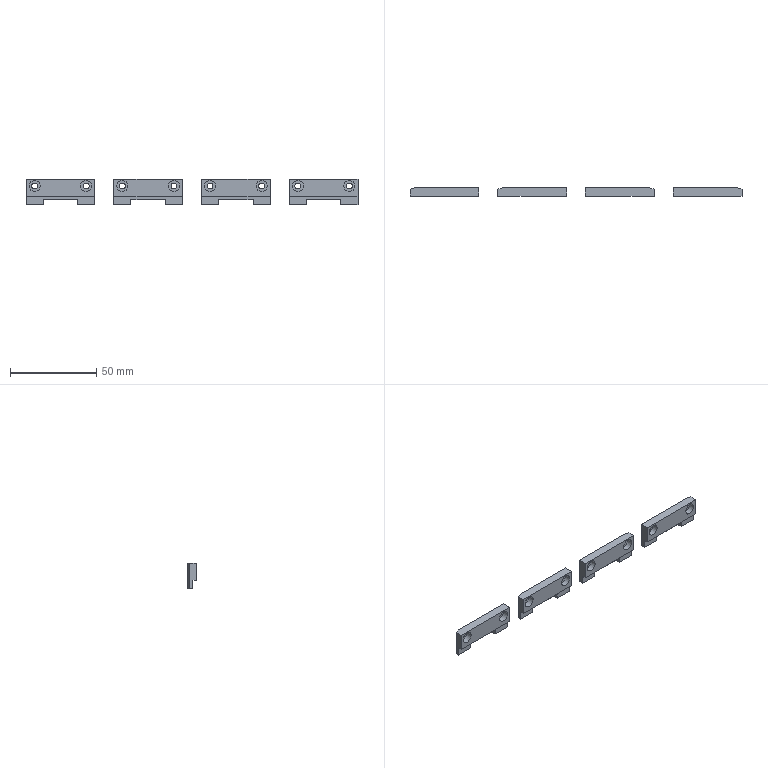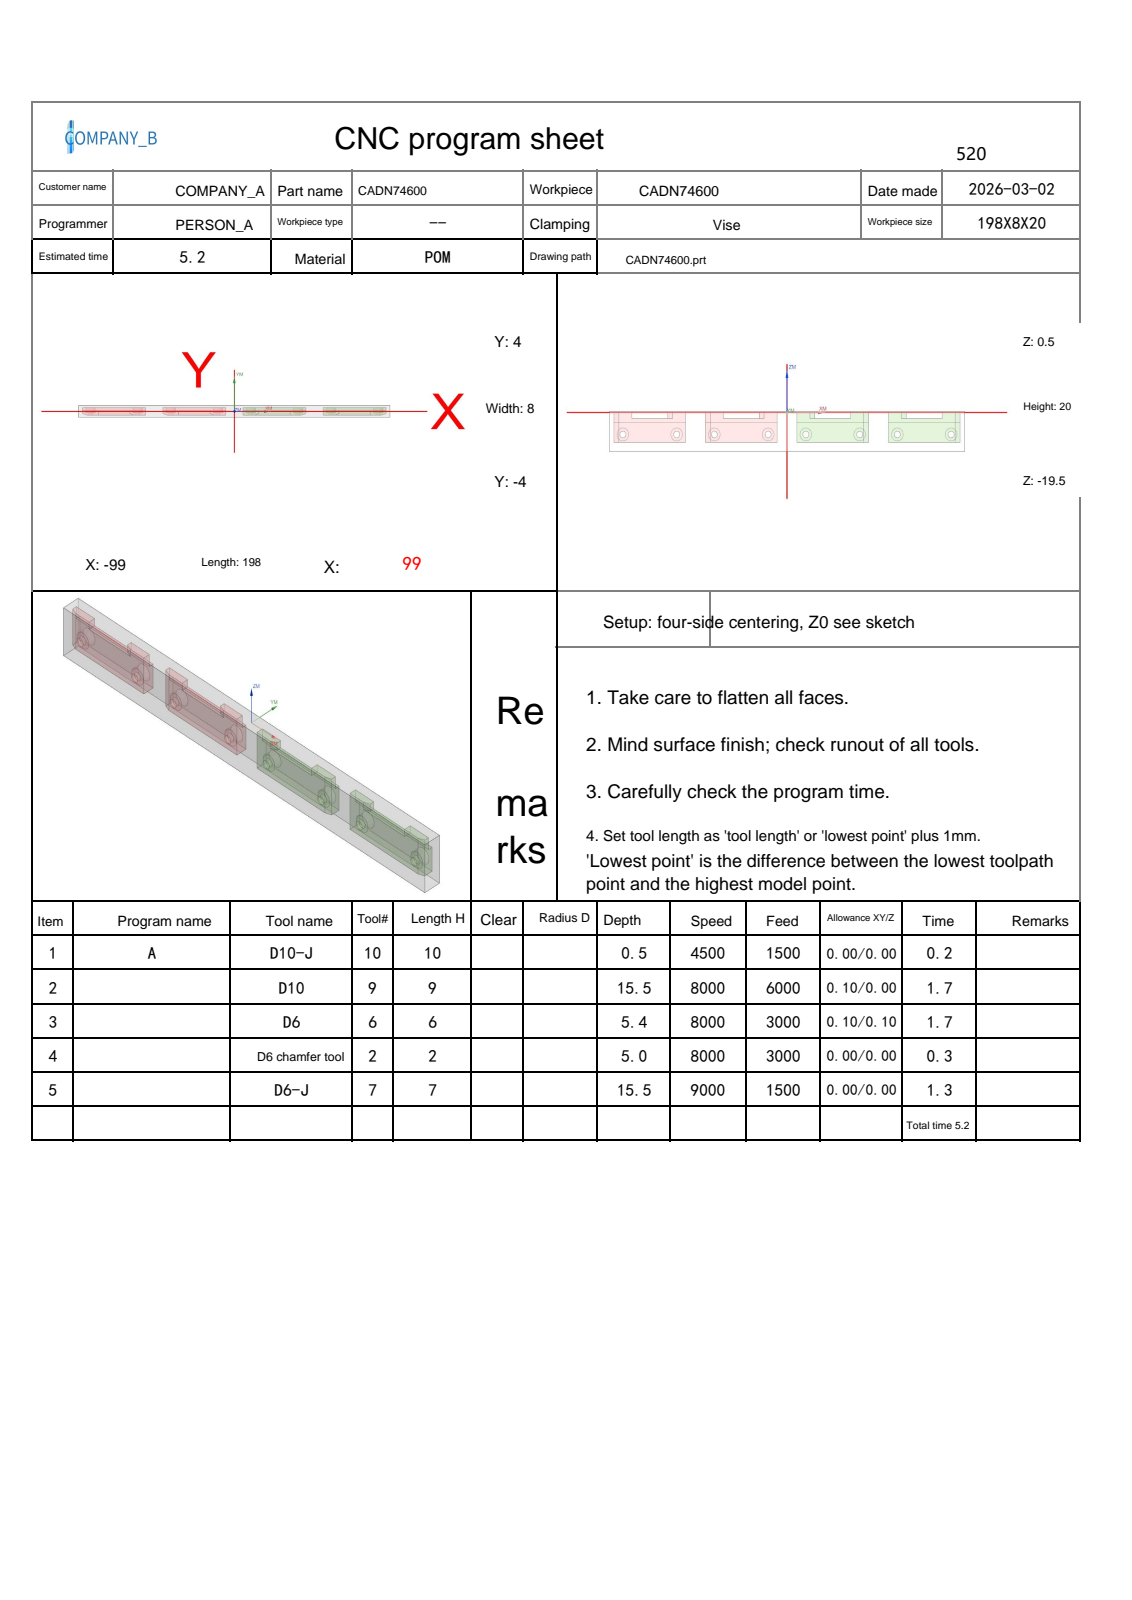NC program | NX | posted by the shop | part box 193 x 5 x 15 mm
Whole program, first 1653 of 2523 lines:
%
O0001
(Machine time: 6.41 MIN)
(===Total Tool:5===)
(T10=D10-J  D=10.  R=0.   D-  H10 Z=0.    )
(T9=D10     D=10.  R=0.   D-  H09 Z=-15.  )
(T6=D6      D=6.   R=0.   D-  H06 Z=-4.9  )
(T2=D6 chamfer tool   D=6.   R=0.   D-  H02 Z=-4.5  )
(T7=D6-J    D=6.   R=0.   D7  H07 Z=-15.  )
G80 G90 G17 G49 G40
G91 G28 Z0
M01
N1 T10 M06
(D10-J  D=10. R=0. H=10 ce=0.00 di=0.00)
G00 G90 G54 X106.5 Y0.0 M03 S4500
G43 H10 Z30.
M08
Z2.
G01 Z0.0 F1500.
X101.5
X-101.5
X-106.5
Z2.
G00 Z30.
G91 G28 Z0.0
M05
M09
G91 G28 Z0.0
M01
N2 T09 M06
(D10  D=10. R=0. H=09 ce=0.10 di=0.00)
G00 G90 G54 X76.5 Y7.6 M03 S8000
G43 H09 Z30.
M08
Z.5
G01 X96.5 Z.372 F6000.
G02 X101.6 Y2.5 Z.321 I0.0 J-5.1
G01 Y-1.5 Z.295
G02 X98.244 Y-6.292 Z.256 I-5.1 J0.0
G01 X95.497 Y-7.292 Z.237
G02 X93.753 Y-7.6 Z.225 I-1.744 J4.792
G01 X56.5 Z-.013
G02 X51.4 Y-2.5 Z-.064 I0.0 J5.1
G01 Y2.5 Z-.096
G02 X56.5 Y7.6 Z-.147 I5.1 J0.0
G01 X96.5 Z-.403
G02 X101.6 Y2.5 Z-.454 I0.0 J-5.1
G01 Y-1.5 Z-.48
G02 X98.244 Y-6.292 Z-.519 I-5.1 J0.0
G01 X95.497 Y-7.292 Z-.538
G02 X93.753 Y-7.6 Z-.55 I-1.744 J4.792
G01 X56.5 Z-.788
G02 X51.4 Y-2.5 Z-.839 I0.0 J5.1
G01 Y2.5 Z-.871
G02 X56.5 Y7.6 Z-.922 I5.1 J0.0
G01 X96.5 Z-1.178
G02 X101.6 Y2.5 Z-1.229 I0.0 J-5.1
G01 Y-1.5 Z-1.255
G02 X98.244 Y-6.292 Z-1.294 I-5.1 J0.0
G01 X95.497 Y-7.292 Z-1.313
G02 X93.753 Y-7.6 Z-1.325 I-1.744 J4.792
G01 X56.5 Z-1.563
G02 X51.4 Y-2.5 Z-1.614 I0.0 J5.1
G01 Y2.5 Z-1.646
G02 X56.5 Y7.6 Z-1.697 I5.1 J0.0
G01 X96.5 Z-1.953
G02 X101.6 Y2.5 Z-2.004 I0.0 J-5.1
G01 Y-1.5 Z-2.03
G02 X98.244 Y-6.292 Z-2.069 I-5.1 J0.0
G01 X95.497 Y-7.292 Z-2.088
G02 X93.753 Y-7.6 Z-2.1 I-1.744 J4.792
G01 X56.5 Z-2.338
G02 X51.4 Y-2.5 Z-2.389 I0.0 J5.1
G01 Y2.5 Z-2.421
G02 X56.5 Y7.6 Z-2.472 I5.1 J0.0
G01 X96.5 Z-2.728
G02 X101.6 Y2.5 Z-2.779 I0.0 J-5.1
G01 Y-1.5 Z-2.805
G02 X98.244 Y-6.292 Z-2.844 I-5.1 J0.0
G01 X95.497 Y-7.292 Z-2.863
G02 X93.753 Y-7.6 Z-2.875 I-1.744 J4.792
G01 X56.5 Z-3.113
G02 X51.4 Y-2.5 Z-3.164 I0.0 J5.1
G01 Y2.5 Z-3.196
G02 X56.5 Y7.6 Z-3.247 I5.1 J0.0
G01 X96.5 Z-3.503
G02 X101.6 Y2.5 Z-3.554 I0.0 J-5.1
G01 Y-1.5 Z-3.58
G02 X98.244 Y-6.292 Z-3.619 I-5.1 J0.0
G01 X95.497 Y-7.292 Z-3.638
G02 X93.753 Y-7.6 Z-3.65 I-1.744 J4.792
G01 X56.5 Z-3.888
G02 X51.4 Y-2.5 Z-3.939 I0.0 J5.1
G01 Y2.5 Z-3.971
G02 X56.5 Y7.6 Z-4.022 I5.1 J0.0
G01 X96.5 Z-4.278
G02 X101.6 Y2.5 Z-4.329 I0.0 J-5.1
G01 Y-1.5 Z-4.355
G02 X98.244 Y-6.292 Z-4.394 I-5.1 J0.0
G01 X95.497 Y-7.292 Z-4.413
G02 X93.753 Y-7.6 Z-4.425 I-1.744 J4.792
G01 X56.5 Z-4.663
G02 X51.4 Y-2.5 Z-4.714 I0.0 J5.1
G01 Y2.5 Z-4.746
G02 X56.5 Y7.6 Z-4.797 I5.1 J0.0
G01 X96.5 Z-5.053
G02 X101.6 Y2.5 Z-5.104 I0.0 J-5.1
G01 Y-1.5 Z-5.13
G02 X98.244 Y-6.292 Z-5.169 I-5.1 J0.0
G01 X95.497 Y-7.292 Z-5.188
G02 X93.753 Y-7.6 Z-5.2 I-1.744 J4.792
G01 X56.5 Z-5.438
G02 X51.4 Y-2.5 Z-5.489 I0.0 J5.1
G01 Y2.5 Z-5.521
G02 X56.5 Y7.6 Z-5.572 I5.1 J0.0
G01 X96.5 Z-5.828
G02 X101.6 Y2.5 Z-5.879 I0.0 J-5.1
G01 Y-1.5 Z-5.905
G02 X98.244 Y-6.292 Z-5.944 I-5.1 J0.0
G01 X95.497 Y-7.292 Z-5.963
G02 X93.753 Y-7.6 Z-5.975 I-1.744 J4.792
G01 X56.5 Z-6.213
G02 X51.4 Y-2.5 Z-6.264 I0.0 J5.1
G01 Y2.5 Z-6.296
G02 X56.5 Y7.6 Z-6.347 I5.1 J0.0
G01 X96.5 Z-6.603
G02 X101.6 Y2.5 Z-6.654 I0.0 J-5.1
G01 Y-1.5 Z-6.68
G02 X98.244 Y-6.292 Z-6.719 I-5.1 J0.0
G01 X95.497 Y-7.292 Z-6.738
G02 X93.753 Y-7.6 Z-6.75 I-1.744 J4.792
G01 X56.5 Z-6.988
G02 X51.4 Y-2.5 Z-7.039 I0.0 J5.1
G01 Y2.5 Z-7.071
G02 X56.5 Y7.6 Z-7.122 I5.1 J0.0
G01 X96.5 Z-7.378
G02 X101.6 Y2.5 Z-7.429 I0.0 J-5.1
G01 Y-1.5 Z-7.455
G02 X98.244 Y-6.292 Z-7.494 I-5.1 J0.0
G01 X95.497 Y-7.292 Z-7.513
G02 X93.753 Y-7.6 Z-7.525 I-1.744 J4.792
G01 X56.5 Z-7.763
G02 X51.4 Y-2.5 Z-7.814 I0.0 J5.1
G01 Y2.5 Z-7.846
G02 X56.5 Y7.6 Z-7.897 I5.1 J0.0
G01 X96.5 Z-8.153
G02 X101.6 Y2.5 Z-8.204 I0.0 J-5.1
G01 Y-1.5 Z-8.23
G02 X98.244 Y-6.292 Z-8.269 I-5.1 J0.0
G01 X95.497 Y-7.292 Z-8.288
G02 X93.753 Y-7.6 Z-8.3 I-1.744 J4.792
G01 X56.5 Z-8.538
G02 X51.4 Y-2.5 Z-8.589 I0.0 J5.1
G01 Y2.5 Z-8.621
G02 X56.5 Y7.6 Z-8.672 I5.1 J0.0
G01 X96.5 Z-8.928
G02 X101.6 Y2.5 Z-8.979 I0.0 J-5.1
G01 Y-1.5 Z-9.005
G02 X98.244 Y-6.292 Z-9.044 I-5.1 J0.0
G01 X95.497 Y-7.292 Z-9.063
G02 X93.753 Y-7.6 Z-9.075 I-1.744 J4.792
G01 X56.5 Z-9.313
G02 X51.4 Y-2.5 Z-9.364 I0.0 J5.1
G01 Y2.5 Z-9.396
G02 X56.5 Y7.6 Z-9.447 I5.1 J0.0
G01 X96.5 Z-9.703
G02 X101.6 Y2.5 Z-9.754 I0.0 J-5.1
G01 Y-1.5 Z-9.78
G02 X98.244 Y-6.292 Z-9.819 I-5.1 J0.0
G01 X95.497 Y-7.292 Z-9.838
G02 X93.753 Y-7.6 Z-9.85 I-1.744 J4.792
G01 X56.5 Z-10.088
G02 X51.4 Y-2.5 Z-10.139 I0.0 J5.1
G01 Y2.5 Z-10.171
G02 X56.5 Y7.6 Z-10.222 I5.1 J0.0
G01 X96.5 Z-10.478
G02 X101.6 Y2.5 Z-10.529 I0.0 J-5.1
G01 Y-1.5 Z-10.555
G02 X98.244 Y-6.292 Z-10.594 I-5.1 J0.0
G01 X95.497 Y-7.292 Z-10.613
G02 X93.753 Y-7.6 Z-10.625 I-1.744 J4.792
G01 X56.5 Z-10.863
G02 X51.4 Y-2.5 Z-10.914 I0.0 J5.1
G01 Y2.5 Z-10.946
G02 X56.5 Y7.6 Z-10.997 I5.1 J0.0
G01 X96.5 Z-11.253
G02 X101.6 Y2.5 Z-11.304 I0.0 J-5.1
G01 Y-1.5 Z-11.33
G02 X98.244 Y-6.292 Z-11.369 I-5.1 J0.0
G01 X95.497 Y-7.292 Z-11.388
G02 X93.753 Y-7.6 Z-11.4 I-1.744 J4.792
G01 X56.5 Z-11.638
G02 X51.4 Y-2.5 Z-11.689 I0.0 J5.1
G01 Y2.5 Z-11.721
G02 X56.5 Y7.6 Z-11.772 I5.1 J0.0
G01 X96.5 Z-12.028
G02 X101.6 Y2.5 Z-12.079 I0.0 J-5.1
G01 Y-1.5 Z-12.105
G02 X98.244 Y-6.292 Z-12.144 I-5.1 J0.0
G01 X95.497 Y-7.292 Z-12.163
G02 X93.753 Y-7.6 Z-12.175 I-1.744 J4.792
G01 X56.5 Z-12.413
G02 X51.4 Y-2.5 Z-12.464 I0.0 J5.1
G01 Y2.5 Z-12.496
G02 X56.5 Y7.6 Z-12.547 I5.1 J0.0
G01 X96.5 Z-12.803
G02 X101.6 Y2.5 Z-12.854 I0.0 J-5.1
G01 Y-1.5 Z-12.88
G02 X98.244 Y-6.292 Z-12.919 I-5.1 J0.0
G01 X95.497 Y-7.292 Z-12.938
G02 X93.753 Y-7.6 Z-12.95 I-1.744 J4.792
G01 X56.5 Z-13.188
G02 X51.4 Y-2.5 Z-13.239 I0.0 J5.1
G01 Y2.5 Z-13.271
G02 X56.5 Y7.6 Z-13.322 I5.1 J0.0
G01 X96.5 Z-13.578
G02 X101.6 Y2.5 Z-13.629 I0.0 J-5.1
G01 Y-1.5 Z-13.655
G02 X98.244 Y-6.292 Z-13.694 I-5.1 J0.0
G01 X95.497 Y-7.292 Z-13.713
G02 X93.753 Y-7.6 Z-13.725 I-1.744 J4.792
G01 X56.5 Z-13.963
G02 X51.4 Y-2.5 Z-14.014 I0.0 J5.1
G01 Y2.5 Z-14.046
G02 X56.5 Y7.6 Z-14.097 I5.1 J0.0
G01 X96.5 Z-14.353
G02 X101.6 Y2.5 Z-14.404 I0.0 J-5.1
G01 Y-1.5 Z-14.43
G02 X98.244 Y-6.292 Z-14.469 I-5.1 J0.0
G01 X95.497 Y-7.292 Z-14.488
G02 X93.753 Y-7.6 Z-14.5 I-1.744 J4.792
G01 X56.5 Z-14.738
G02 X51.4 Y-2.5 Z-14.789 I0.0 J5.1
G01 Y2.5 Z-14.821
G02 X56.5 Y7.6 Z-14.872 I5.1 J0.0
G01 X76.5 Z-15.
X96.5
G02 X101.6 Y2.5 I0.0 J-5.1
G01 Y-1.5
G02 X98.244 Y-6.292 I-5.1 J0.0
G01 X95.497 Y-7.292
G02 X93.753 Y-7.6 I-1.744 J4.792
G01 X56.5
G02 X51.4 Y-2.5 I0.0 J5.1
G01 Y2.5
G02 X56.5 Y7.6 I5.1 J0.0
G01 X76.5
X77.
Z-14.
G00 Z30.
X25.5
Z.5
G01 X45.5 Z.372
G02 X50.6 Y2.5 Z.321 I0.0 J-5.1
G01 Y-1.5 Z.295
G02 X47.244 Y-6.292 Z.256 I-5.1 J0.0
G01 X44.497 Y-7.292 Z.237
G02 X42.753 Y-7.6 Z.225 I-1.744 J4.792
G01 X5.5 Z-.013
G02 X.4 Y-2.5 Z-.064 I0.0 J5.1
G01 Y2.5 Z-.096
G02 X5.5 Y7.6 Z-.147 I5.1 J0.0
G01 X45.5 Z-.403
G02 X50.6 Y2.5 Z-.454 I0.0 J-5.1
G01 Y-1.5 Z-.48
G02 X47.244 Y-6.292 Z-.519 I-5.1 J0.0
G01 X44.497 Y-7.292 Z-.538
G02 X42.753 Y-7.6 Z-.55 I-1.744 J4.792
G01 X5.5 Z-.788
G02 X.4 Y-2.5 Z-.839 I0.0 J5.1
G01 Y2.5 Z-.871
G02 X5.5 Y7.6 Z-.922 I5.1 J0.0
G01 X45.5 Z-1.178
G02 X50.6 Y2.5 Z-1.229 I0.0 J-5.1
G01 Y-1.5 Z-1.255
G02 X47.244 Y-6.292 Z-1.294 I-5.1 J0.0
G01 X44.497 Y-7.292 Z-1.313
G02 X42.753 Y-7.6 Z-1.325 I-1.744 J4.792
G01 X5.5 Z-1.563
G02 X.4 Y-2.5 Z-1.614 I0.0 J5.1
G01 Y2.5 Z-1.646
G02 X5.5 Y7.6 Z-1.697 I5.1 J0.0
G01 X45.5 Z-1.953
G02 X50.6 Y2.5 Z-2.004 I0.0 J-5.1
G01 Y-1.5 Z-2.03
G02 X47.244 Y-6.292 Z-2.069 I-5.1 J0.0
G01 X44.497 Y-7.292 Z-2.088
G02 X42.753 Y-7.6 Z-2.1 I-1.744 J4.792
G01 X5.5 Z-2.338
G02 X.4 Y-2.5 Z-2.389 I0.0 J5.1
G01 Y2.5 Z-2.421
G02 X5.5 Y7.6 Z-2.472 I5.1 J0.0
G01 X45.5 Z-2.728
G02 X50.6 Y2.5 Z-2.779 I0.0 J-5.1
G01 Y-1.5 Z-2.805
G02 X47.244 Y-6.292 Z-2.844 I-5.1 J0.0
G01 X44.497 Y-7.292 Z-2.863
G02 X42.753 Y-7.6 Z-2.875 I-1.744 J4.792
G01 X5.5 Z-3.113
G02 X.4 Y-2.5 Z-3.164 I0.0 J5.1
G01 Y2.5 Z-3.196
G02 X5.5 Y7.6 Z-3.247 I5.1 J0.0
G01 X45.5 Z-3.503
G02 X50.6 Y2.5 Z-3.554 I0.0 J-5.1
G01 Y-1.5 Z-3.58
G02 X47.244 Y-6.292 Z-3.619 I-5.1 J0.0
G01 X44.497 Y-7.292 Z-3.638
G02 X42.753 Y-7.6 Z-3.65 I-1.744 J4.792
G01 X5.5 Z-3.888
G02 X.4 Y-2.5 Z-3.939 I0.0 J5.1
G01 Y2.5 Z-3.971
G02 X5.5 Y7.6 Z-4.022 I5.1 J0.0
G01 X45.5 Z-4.278
G02 X50.6 Y2.5 Z-4.329 I0.0 J-5.1
G01 Y-1.5 Z-4.355
G02 X47.244 Y-6.292 Z-4.394 I-5.1 J0.0
G01 X44.497 Y-7.292 Z-4.413
G02 X42.753 Y-7.6 Z-4.425 I-1.744 J4.792
G01 X5.5 Z-4.663
G02 X.4 Y-2.5 Z-4.714 I0.0 J5.1
G01 Y2.5 Z-4.746
G02 X5.5 Y7.6 Z-4.797 I5.1 J0.0
G01 X45.5 Z-5.053
G02 X50.6 Y2.5 Z-5.104 I0.0 J-5.1
G01 Y-1.5 Z-5.13
G02 X47.244 Y-6.292 Z-5.169 I-5.1 J0.0
G01 X44.497 Y-7.292 Z-5.188
G02 X42.753 Y-7.6 Z-5.2 I-1.744 J4.792
G01 X5.5 Z-5.438
G02 X.4 Y-2.5 Z-5.489 I0.0 J5.1
G01 Y2.5 Z-5.521
G02 X5.5 Y7.6 Z-5.572 I5.1 J0.0
G01 X45.5 Z-5.828
G02 X50.6 Y2.5 Z-5.879 I0.0 J-5.1
G01 Y-1.5 Z-5.905
G02 X47.244 Y-6.292 Z-5.944 I-5.1 J0.0
G01 X44.497 Y-7.292 Z-5.963
G02 X42.753 Y-7.6 Z-5.975 I-1.744 J4.792
G01 X5.5 Z-6.213
G02 X.4 Y-2.5 Z-6.264 I0.0 J5.1
G01 Y2.5 Z-6.296
G02 X5.5 Y7.6 Z-6.347 I5.1 J0.0
G01 X45.5 Z-6.603
G02 X50.6 Y2.5 Z-6.654 I0.0 J-5.1
G01 Y-1.5 Z-6.68
G02 X47.244 Y-6.292 Z-6.719 I-5.1 J0.0
G01 X44.497 Y-7.292 Z-6.738
G02 X42.753 Y-7.6 Z-6.75 I-1.744 J4.792
G01 X5.5 Z-6.988
G02 X.4 Y-2.5 Z-7.039 I0.0 J5.1
G01 Y2.5 Z-7.071
G02 X5.5 Y7.6 Z-7.122 I5.1 J0.0
G01 X45.5 Z-7.378
G02 X50.6 Y2.5 Z-7.429 I0.0 J-5.1
G01 Y-1.5 Z-7.455
G02 X47.244 Y-6.292 Z-7.494 I-5.1 J0.0
G01 X44.497 Y-7.292 Z-7.513
G02 X42.753 Y-7.6 Z-7.525 I-1.744 J4.792
G01 X5.5 Z-7.763
G02 X.4 Y-2.5 Z-7.814 I0.0 J5.1
G01 Y2.5 Z-7.846
G02 X5.5 Y7.6 Z-7.897 I5.1 J0.0
G01 X45.5 Z-8.153
G02 X50.6 Y2.5 Z-8.204 I0.0 J-5.1
G01 Y-1.5 Z-8.23
G02 X47.244 Y-6.292 Z-8.269 I-5.1 J0.0
G01 X44.497 Y-7.292 Z-8.288
G02 X42.753 Y-7.6 Z-8.3 I-1.744 J4.792
G01 X5.5 Z-8.538
G02 X.4 Y-2.5 Z-8.589 I0.0 J5.1
G01 Y2.5 Z-8.621
G02 X5.5 Y7.6 Z-8.672 I5.1 J0.0
G01 X45.5 Z-8.928
G02 X50.6 Y2.5 Z-8.979 I0.0 J-5.1
G01 Y-1.5 Z-9.005
G02 X47.244 Y-6.292 Z-9.044 I-5.1 J0.0
G01 X44.497 Y-7.292 Z-9.063
G02 X42.753 Y-7.6 Z-9.075 I-1.744 J4.792
G01 X5.5 Z-9.313
G02 X.4 Y-2.5 Z-9.364 I0.0 J5.1
G01 Y2.5 Z-9.396
G02 X5.5 Y7.6 Z-9.447 I5.1 J0.0
G01 X45.5 Z-9.703
G02 X50.6 Y2.5 Z-9.754 I0.0 J-5.1
G01 Y-1.5 Z-9.78
G02 X47.244 Y-6.292 Z-9.819 I-5.1 J0.0
G01 X44.497 Y-7.292 Z-9.838
G02 X42.753 Y-7.6 Z-9.85 I-1.744 J4.792
G01 X5.5 Z-10.088
G02 X.4 Y-2.5 Z-10.139 I0.0 J5.1
G01 Y2.5 Z-10.171
G02 X5.5 Y7.6 Z-10.222 I5.1 J0.0
G01 X45.5 Z-10.478
G02 X50.6 Y2.5 Z-10.529 I0.0 J-5.1
G01 Y-1.5 Z-10.555
G02 X47.244 Y-6.292 Z-10.594 I-5.1 J0.0
G01 X44.497 Y-7.292 Z-10.613
G02 X42.753 Y-7.6 Z-10.625 I-1.744 J4.792
G01 X5.5 Z-10.863
G02 X.4 Y-2.5 Z-10.914 I0.0 J5.1
G01 Y2.5 Z-10.946
G02 X5.5 Y7.6 Z-10.997 I5.1 J0.0
G01 X45.5 Z-11.253
G02 X50.6 Y2.5 Z-11.304 I0.0 J-5.1
G01 Y-1.5 Z-11.33
G02 X47.244 Y-6.292 Z-11.369 I-5.1 J0.0
G01 X44.497 Y-7.292 Z-11.388
G02 X42.753 Y-7.6 Z-11.4 I-1.744 J4.792
G01 X5.5 Z-11.638
G02 X.4 Y-2.5 Z-11.689 I0.0 J5.1
G01 Y2.5 Z-11.721
G02 X5.5 Y7.6 Z-11.772 I5.1 J0.0
G01 X45.5 Z-12.028
G02 X50.6 Y2.5 Z-12.079 I0.0 J-5.1
G01 Y-1.5 Z-12.105
G02 X47.244 Y-6.292 Z-12.144 I-5.1 J0.0
G01 X44.497 Y-7.292 Z-12.163
G02 X42.753 Y-7.6 Z-12.175 I-1.744 J4.792
G01 X5.5 Z-12.413
G02 X.4 Y-2.5 Z-12.464 I0.0 J5.1
G01 Y2.5 Z-12.496
G02 X5.5 Y7.6 Z-12.547 I5.1 J0.0
G01 X45.5 Z-12.803
G02 X50.6 Y2.5 Z-12.854 I0.0 J-5.1
G01 Y-1.5 Z-12.88
G02 X47.244 Y-6.292 Z-12.919 I-5.1 J0.0
G01 X44.497 Y-7.292 Z-12.938
G02 X42.753 Y-7.6 Z-12.95 I-1.744 J4.792
G01 X5.5 Z-13.188
G02 X.4 Y-2.5 Z-13.239 I0.0 J5.1
G01 Y2.5 Z-13.271
G02 X5.5 Y7.6 Z-13.322 I5.1 J0.0
G01 X45.5 Z-13.578
G02 X50.6 Y2.5 Z-13.629 I0.0 J-5.1
G01 Y-1.5 Z-13.655
G02 X47.244 Y-6.292 Z-13.694 I-5.1 J0.0
G01 X44.497 Y-7.292 Z-13.713
G02 X42.753 Y-7.6 Z-13.725 I-1.744 J4.792
G01 X5.5 Z-13.963
G02 X.4 Y-2.5 Z-14.014 I0.0 J5.1
G01 Y2.5 Z-14.046
G02 X5.5 Y7.6 Z-14.097 I5.1 J0.0
G01 X45.5 Z-14.353
G02 X50.6 Y2.5 Z-14.404 I0.0 J-5.1
G01 Y-1.5 Z-14.43
G02 X47.244 Y-6.292 Z-14.469 I-5.1 J0.0
G01 X44.497 Y-7.292 Z-14.488
G02 X42.753 Y-7.6 Z-14.5 I-1.744 J4.792
G01 X5.5 Z-14.738
G02 X.4 Y-2.5 Z-14.789 I0.0 J5.1
G01 Y2.5 Z-14.821
G02 X5.5 Y7.6 Z-14.872 I5.1 J0.0
G01 X25.5 Z-15.
X45.5
G02 X50.6 Y2.5 I0.0 J-5.1
G01 Y-1.5
G02 X47.244 Y-6.292 I-5.1 J0.0
G01 X44.497 Y-7.292
G02 X42.753 Y-7.6 I-1.744 J4.792
G01 X5.5
G02 X.4 Y-2.5 I0.0 J5.1
G01 Y2.5
G02 X5.5 Y7.6 I5.1 J0.0
G01 X25.5
X26.
Z-14.
G00 Z30.
X-25.5
Z.5
G01 X-5.5 Z.372
G02 X-.4 Y2.5 Z.321 I0.0 J-5.1
G01 Y-2.5 Z.289
G02 X-5.5 Y-7.6 Z.238 I-5.1 J0.0
G01 X-42.753 Z0.0
G02 X-44.497 Y-7.292 Z-.012 I0.0 J5.1
G01 X-47.244 Y-6.292 Z-.031
G02 X-50.6 Y-1.5 Z-.07 I1.744 J4.792
G01 Y2.5 Z-.096
G02 X-45.5 Y7.6 Z-.147 I5.1 J0.0
G01 X-5.5 Z-.403
G02 X-.4 Y2.5 Z-.454 I0.0 J-5.1
G01 Y-2.5 Z-.486
G02 X-5.5 Y-7.6 Z-.537 I-5.1 J0.0
G01 X-42.753 Z-.775
G02 X-44.497 Y-7.292 Z-.787 I0.0 J5.1
G01 X-47.244 Y-6.292 Z-.806
G02 X-50.6 Y-1.5 Z-.845 I1.744 J4.792
G01 Y2.5 Z-.871
G02 X-45.5 Y7.6 Z-.922 I5.1 J0.0
G01 X-5.5 Z-1.178
G02 X-.4 Y2.5 Z-1.229 I0.0 J-5.1
G01 Y-2.5 Z-1.261
G02 X-5.5 Y-7.6 Z-1.312 I-5.1 J0.0
G01 X-42.753 Z-1.55
G02 X-44.497 Y-7.292 Z-1.562 I0.0 J5.1
G01 X-47.244 Y-6.292 Z-1.581
G02 X-50.6 Y-1.5 Z-1.62 I1.744 J4.792
G01 Y2.5 Z-1.646
G02 X-45.5 Y7.6 Z-1.697 I5.1 J0.0
G01 X-5.5 Z-1.953
G02 X-.4 Y2.5 Z-2.004 I0.0 J-5.1
G01 Y-2.5 Z-2.036
G02 X-5.5 Y-7.6 Z-2.087 I-5.1 J0.0
G01 X-42.753 Z-2.325
G02 X-44.497 Y-7.292 Z-2.337 I0.0 J5.1
G01 X-47.244 Y-6.292 Z-2.356
G02 X-50.6 Y-1.5 Z-2.395 I1.744 J4.792
G01 Y2.5 Z-2.421
G02 X-45.5 Y7.6 Z-2.472 I5.1 J0.0
G01 X-5.5 Z-2.728
G02 X-.4 Y2.5 Z-2.779 I0.0 J-5.1
G01 Y-2.5 Z-2.811
G02 X-5.5 Y-7.6 Z-2.862 I-5.1 J0.0
G01 X-42.753 Z-3.1
G02 X-44.497 Y-7.292 Z-3.112 I0.0 J5.1
G01 X-47.244 Y-6.292 Z-3.131
G02 X-50.6 Y-1.5 Z-3.17 I1.744 J4.792
G01 Y2.5 Z-3.196
G02 X-45.5 Y7.6 Z-3.247 I5.1 J0.0
G01 X-5.5 Z-3.503
G02 X-.4 Y2.5 Z-3.554 I0.0 J-5.1
G01 Y-2.5 Z-3.586
G02 X-5.5 Y-7.6 Z-3.637 I-5.1 J0.0
G01 X-42.753 Z-3.875
G02 X-44.497 Y-7.292 Z-3.887 I0.0 J5.1
G01 X-47.244 Y-6.292 Z-3.906
G02 X-50.6 Y-1.5 Z-3.945 I1.744 J4.792
G01 Y2.5 Z-3.971
G02 X-45.5 Y7.6 Z-4.022 I5.1 J0.0
G01 X-5.5 Z-4.278
G02 X-.4 Y2.5 Z-4.329 I0.0 J-5.1
G01 Y-2.5 Z-4.361
G02 X-5.5 Y-7.6 Z-4.412 I-5.1 J0.0
G01 X-42.753 Z-4.65
G02 X-44.497 Y-7.292 Z-4.662 I0.0 J5.1
G01 X-47.244 Y-6.292 Z-4.681
G02 X-50.6 Y-1.5 Z-4.72 I1.744 J4.792
G01 Y2.5 Z-4.746
G02 X-45.5 Y7.6 Z-4.797 I5.1 J0.0
G01 X-5.5 Z-5.053
G02 X-.4 Y2.5 Z-5.104 I0.0 J-5.1
G01 Y-2.5 Z-5.136
G02 X-5.5 Y-7.6 Z-5.187 I-5.1 J0.0
G01 X-42.753 Z-5.425
G02 X-44.497 Y-7.292 Z-5.437 I0.0 J5.1
G01 X-47.244 Y-6.292 Z-5.456
G02 X-50.6 Y-1.5 Z-5.495 I1.744 J4.792
G01 Y2.5 Z-5.521
G02 X-45.5 Y7.6 Z-5.572 I5.1 J0.0
G01 X-5.5 Z-5.828
G02 X-.4 Y2.5 Z-5.879 I0.0 J-5.1
G01 Y-2.5 Z-5.911
G02 X-5.5 Y-7.6 Z-5.962 I-5.1 J0.0
G01 X-42.753 Z-6.2
G02 X-44.497 Y-7.292 Z-6.212 I0.0 J5.1
G01 X-47.244 Y-6.292 Z-6.231
G02 X-50.6 Y-1.5 Z-6.27 I1.744 J4.792
G01 Y2.5 Z-6.296
G02 X-45.5 Y7.6 Z-6.347 I5.1 J0.0
G01 X-5.5 Z-6.603
G02 X-.4 Y2.5 Z-6.654 I0.0 J-5.1
G01 Y-2.5 Z-6.686
G02 X-5.5 Y-7.6 Z-6.737 I-5.1 J0.0
G01 X-42.753 Z-6.975
G02 X-44.497 Y-7.292 Z-6.987 I0.0 J5.1
G01 X-47.244 Y-6.292 Z-7.006
G02 X-50.6 Y-1.5 Z-7.045 I1.744 J4.792
G01 Y2.5 Z-7.071
G02 X-45.5 Y7.6 Z-7.122 I5.1 J0.0
G01 X-5.5 Z-7.378
G02 X-.4 Y2.5 Z-7.429 I0.0 J-5.1
G01 Y-2.5 Z-7.461
G02 X-5.5 Y-7.6 Z-7.512 I-5.1 J0.0
G01 X-42.753 Z-7.75
G02 X-44.497 Y-7.292 Z-7.762 I0.0 J5.1
G01 X-47.244 Y-6.292 Z-7.781
G02 X-50.6 Y-1.5 Z-7.82 I1.744 J4.792
G01 Y2.5 Z-7.846
G02 X-45.5 Y7.6 Z-7.897 I5.1 J0.0
G01 X-5.5 Z-8.153
G02 X-.4 Y2.5 Z-8.204 I0.0 J-5.1
G01 Y-2.5 Z-8.236
G02 X-5.5 Y-7.6 Z-8.287 I-5.1 J0.0
G01 X-42.753 Z-8.525
G02 X-44.497 Y-7.292 Z-8.537 I0.0 J5.1
G01 X-47.244 Y-6.292 Z-8.556
G02 X-50.6 Y-1.5 Z-8.595 I1.744 J4.792
G01 Y2.5 Z-8.621
G02 X-45.5 Y7.6 Z-8.672 I5.1 J0.0
G01 X-5.5 Z-8.928
G02 X-.4 Y2.5 Z-8.979 I0.0 J-5.1
G01 Y-2.5 Z-9.011
G02 X-5.5 Y-7.6 Z-9.062 I-5.1 J0.0
G01 X-42.753 Z-9.3
G02 X-44.497 Y-7.292 Z-9.312 I0.0 J5.1
G01 X-47.244 Y-6.292 Z-9.331
G02 X-50.6 Y-1.5 Z-9.37 I1.744 J4.792
G01 Y2.5 Z-9.396
G02 X-45.5 Y7.6 Z-9.447 I5.1 J0.0
G01 X-5.5 Z-9.703
G02 X-.4 Y2.5 Z-9.754 I0.0 J-5.1
G01 Y-2.5 Z-9.786
G02 X-5.5 Y-7.6 Z-9.837 I-5.1 J0.0
G01 X-42.753 Z-10.075
G02 X-44.497 Y-7.292 Z-10.087 I0.0 J5.1
G01 X-47.244 Y-6.292 Z-10.106
G02 X-50.6 Y-1.5 Z-10.145 I1.744 J4.792
G01 Y2.5 Z-10.171
G02 X-45.5 Y7.6 Z-10.222 I5.1 J0.0
G01 X-5.5 Z-10.478
G02 X-.4 Y2.5 Z-10.529 I0.0 J-5.1
G01 Y-2.5 Z-10.561
G02 X-5.5 Y-7.6 Z-10.612 I-5.1 J0.0
G01 X-42.753 Z-10.85
G02 X-44.497 Y-7.292 Z-10.862 I0.0 J5.1
G01 X-47.244 Y-6.292 Z-10.881
G02 X-50.6 Y-1.5 Z-10.92 I1.744 J4.792
G01 Y2.5 Z-10.946
G02 X-45.5 Y7.6 Z-10.997 I5.1 J0.0
G01 X-5.5 Z-11.253
G02 X-.4 Y2.5 Z-11.304 I0.0 J-5.1
G01 Y-2.5 Z-11.336
G02 X-5.5 Y-7.6 Z-11.387 I-5.1 J0.0
G01 X-42.753 Z-11.625
G02 X-44.497 Y-7.292 Z-11.637 I0.0 J5.1
G01 X-47.244 Y-6.292 Z-11.656
G02 X-50.6 Y-1.5 Z-11.695 I1.744 J4.792
G01 Y2.5 Z-11.721
G02 X-45.5 Y7.6 Z-11.772 I5.1 J0.0
G01 X-5.5 Z-12.028
G02 X-.4 Y2.5 Z-12.079 I0.0 J-5.1
G01 Y-2.5 Z-12.111
G02 X-5.5 Y-7.6 Z-12.162 I-5.1 J0.0
G01 X-42.753 Z-12.4
G02 X-44.497 Y-7.292 Z-12.412 I0.0 J5.1
G01 X-47.244 Y-6.292 Z-12.431
G02 X-50.6 Y-1.5 Z-12.47 I1.744 J4.792
G01 Y2.5 Z-12.496
G02 X-45.5 Y7.6 Z-12.547 I5.1 J0.0
G01 X-5.5 Z-12.803
G02 X-.4 Y2.5 Z-12.854 I0.0 J-5.1
G01 Y-2.5 Z-12.886
G02 X-5.5 Y-7.6 Z-12.937 I-5.1 J0.0
G01 X-42.753 Z-13.175
G02 X-44.497 Y-7.292 Z-13.187 I0.0 J5.1
G01 X-47.244 Y-6.292 Z-13.206
G02 X-50.6 Y-1.5 Z-13.245 I1.744 J4.792
G01 Y2.5 Z-13.271
G02 X-45.5 Y7.6 Z-13.322 I5.1 J0.0
G01 X-5.5 Z-13.578
G02 X-.4 Y2.5 Z-13.629 I0.0 J-5.1
G01 Y-2.5 Z-13.661
G02 X-5.5 Y-7.6 Z-13.712 I-5.1 J0.0
G01 X-42.753 Z-13.95
G02 X-44.497 Y-7.292 Z-13.962 I0.0 J5.1
G01 X-47.244 Y-6.292 Z-13.981
G02 X-50.6 Y-1.5 Z-14.02 I1.744 J4.792
G01 Y2.5 Z-14.046
G02 X-45.5 Y7.6 Z-14.097 I5.1 J0.0
G01 X-5.5 Z-14.353
G02 X-.4 Y2.5 Z-14.404 I0.0 J-5.1
G01 Y-2.5 Z-14.436
G02 X-5.5 Y-7.6 Z-14.487 I-5.1 J0.0
G01 X-42.753 Z-14.725
G02 X-44.497 Y-7.292 Z-14.737 I0.0 J5.1
G01 X-47.244 Y-6.292 Z-14.756
G02 X-50.6 Y-1.5 Z-14.795 I1.744 J4.792
G01 Y2.5 Z-14.821
G02 X-45.5 Y7.6 Z-14.872 I5.1 J0.0
G01 X-25.5 Z-15.
X-5.5
G02 X-.4 Y2.5 I0.0 J-5.1
G01 Y-2.5
G02 X-5.5 Y-7.6 I-5.1 J0.0
G01 X-42.753
G02 X-44.497 Y-7.292 I0.0 J5.1
G01 X-47.244 Y-6.292
G02 X-50.6 Y-1.5 I1.744 J4.792
G01 Y2.5
G02 X-45.5 Y7.6 I5.1 J0.0
G01 X-25.5
X-25.
Z-14.
G00 Z30.
X-76.5
Z.5
G01 X-56.5 Z.372
G02 X-51.4 Y2.5 Z.321 I0.0 J-5.1
G01 Y-2.5 Z.289
G02 X-56.5 Y-7.6 Z.238 I-5.1 J0.0
G01 X-93.753 Z0.0
G02 X-95.497 Y-7.292 Z-.012 I0.0 J5.1
G01 X-98.244 Y-6.292 Z-.031
G02 X-101.6 Y-1.5 Z-.07 I1.744 J4.792
G01 Y2.5 Z-.096
G02 X-96.5 Y7.6 Z-.147 I5.1 J0.0
G01 X-56.5 Z-.403
G02 X-51.4 Y2.5 Z-.454 I0.0 J-5.1
G01 Y-2.5 Z-.486
G02 X-56.5 Y-7.6 Z-.537 I-5.1 J0.0
G01 X-93.753 Z-.775
G02 X-95.497 Y-7.292 Z-.787 I0.0 J5.1
G01 X-98.244 Y-6.292 Z-.806
G02 X-101.6 Y-1.5 Z-.845 I1.744 J4.792
G01 Y2.5 Z-.871
G02 X-96.5 Y7.6 Z-.922 I5.1 J0.0
G01 X-56.5 Z-1.178
G02 X-51.4 Y2.5 Z-1.229 I0.0 J-5.1
G01 Y-2.5 Z-1.261
G02 X-56.5 Y-7.6 Z-1.312 I-5.1 J0.0
G01 X-93.753 Z-1.55
G02 X-95.497 Y-7.292 Z-1.562 I0.0 J5.1
G01 X-98.244 Y-6.292 Z-1.581
G02 X-101.6 Y-1.5 Z-1.62 I1.744 J4.792
G01 Y2.5 Z-1.646
G02 X-96.5 Y7.6 Z-1.697 I5.1 J0.0
G01 X-56.5 Z-1.953
G02 X-51.4 Y2.5 Z-2.004 I0.0 J-5.1
G01 Y-2.5 Z-2.036
G02 X-56.5 Y-7.6 Z-2.087 I-5.1 J0.0
G01 X-93.753 Z-2.325
G02 X-95.497 Y-7.292 Z-2.337 I0.0 J5.1
G01 X-98.244 Y-6.292 Z-2.356
G02 X-101.6 Y-1.5 Z-2.395 I1.744 J4.792
G01 Y2.5 Z-2.421
G02 X-96.5 Y7.6 Z-2.472 I5.1 J0.0
G01 X-56.5 Z-2.728
G02 X-51.4 Y2.5 Z-2.779 I0.0 J-5.1
G01 Y-2.5 Z-2.811
G02 X-56.5 Y-7.6 Z-2.862 I-5.1 J0.0
G01 X-93.753 Z-3.1
G02 X-95.497 Y-7.292 Z-3.112 I0.0 J5.1
G01 X-98.244 Y-6.292 Z-3.131
G02 X-101.6 Y-1.5 Z-3.17 I1.744 J4.792
G01 Y2.5 Z-3.196
G02 X-96.5 Y7.6 Z-3.247 I5.1 J0.0
G01 X-56.5 Z-3.503
G02 X-51.4 Y2.5 Z-3.554 I0.0 J-5.1
G01 Y-2.5 Z-3.586
G02 X-56.5 Y-7.6 Z-3.637 I-5.1 J0.0
G01 X-93.753 Z-3.875
G02 X-95.497 Y-7.292 Z-3.887 I0.0 J5.1
G01 X-98.244 Y-6.292 Z-3.906
G02 X-101.6 Y-1.5 Z-3.945 I1.744 J4.792
G01 Y2.5 Z-3.971
G02 X-96.5 Y7.6 Z-4.022 I5.1 J0.0
G01 X-56.5 Z-4.278
G02 X-51.4 Y2.5 Z-4.329 I0.0 J-5.1
G01 Y-2.5 Z-4.361
G02 X-56.5 Y-7.6 Z-4.412 I-5.1 J0.0
G01 X-93.753 Z-4.65
G02 X-95.497 Y-7.292 Z-4.662 I0.0 J5.1
G01 X-98.244 Y-6.292 Z-4.681
G02 X-101.6 Y-1.5 Z-4.72 I1.744 J4.792
G01 Y2.5 Z-4.746
G02 X-96.5 Y7.6 Z-4.797 I5.1 J0.0
G01 X-56.5 Z-5.053
G02 X-51.4 Y2.5 Z-5.104 I0.0 J-5.1
G01 Y-2.5 Z-5.136
G02 X-56.5 Y-7.6 Z-5.187 I-5.1 J0.0
G01 X-93.753 Z-5.425
G02 X-95.497 Y-7.292 Z-5.437 I0.0 J5.1
G01 X-98.244 Y-6.292 Z-5.456
G02 X-101.6 Y-1.5 Z-5.495 I1.744 J4.792
G01 Y2.5 Z-5.521
G02 X-96.5 Y7.6 Z-5.572 I5.1 J0.0
G01 X-56.5 Z-5.828
G02 X-51.4 Y2.5 Z-5.879 I0.0 J-5.1
G01 Y-2.5 Z-5.911
G02 X-56.5 Y-7.6 Z-5.962 I-5.1 J0.0
G01 X-93.753 Z-6.2
G02 X-95.497 Y-7.292 Z-6.212 I0.0 J5.1
G01 X-98.244 Y-6.292 Z-6.231
G02 X-101.6 Y-1.5 Z-6.27 I1.744 J4.792
G01 Y2.5 Z-6.296
G02 X-96.5 Y7.6 Z-6.347 I5.1 J0.0
G01 X-56.5 Z-6.603
G02 X-51.4 Y2.5 Z-6.654 I0.0 J-5.1
G01 Y-2.5 Z-6.686
G02 X-56.5 Y-7.6 Z-6.737 I-5.1 J0.0
G01 X-93.753 Z-6.975
G02 X-95.497 Y-7.292 Z-6.987 I0.0 J5.1
G01 X-98.244 Y-6.292 Z-7.006
G02 X-101.6 Y-1.5 Z-7.045 I1.744 J4.792
G01 Y2.5 Z-7.071
G02 X-96.5 Y7.6 Z-7.122 I5.1 J0.0
G01 X-56.5 Z-7.378
G02 X-51.4 Y2.5 Z-7.429 I0.0 J-5.1
G01 Y-2.5 Z-7.461
G02 X-56.5 Y-7.6 Z-7.512 I-5.1 J0.0
G01 X-93.753 Z-7.75
G02 X-95.497 Y-7.292 Z-7.762 I0.0 J5.1
G01 X-98.244 Y-6.292 Z-7.781
G02 X-101.6 Y-1.5 Z-7.82 I1.744 J4.792
G01 Y2.5 Z-7.846
G02 X-96.5 Y7.6 Z-7.897 I5.1 J0.0
G01 X-56.5 Z-8.153
G02 X-51.4 Y2.5 Z-8.204 I0.0 J-5.1
G01 Y-2.5 Z-8.236
G02 X-56.5 Y-7.6 Z-8.287 I-5.1 J0.0
G01 X-93.753 Z-8.525
G02 X-95.497 Y-7.292 Z-8.537 I0.0 J5.1
G01 X-98.244 Y-6.292 Z-8.556
G02 X-101.6 Y-1.5 Z-8.595 I1.744 J4.792
G01 Y2.5 Z-8.621
G02 X-96.5 Y7.6 Z-8.672 I5.1 J0.0
G01 X-56.5 Z-8.928
G02 X-51.4 Y2.5 Z-8.979 I0.0 J-5.1
G01 Y-2.5 Z-9.011
G02 X-56.5 Y-7.6 Z-9.062 I-5.1 J0.0
G01 X-93.753 Z-9.3
G02 X-95.497 Y-7.292 Z-9.312 I0.0 J5.1
G01 X-98.244 Y-6.292 Z-9.331
G02 X-101.6 Y-1.5 Z-9.37 I1.744 J4.792
G01 Y2.5 Z-9.396
G02 X-96.5 Y7.6 Z-9.447 I5.1 J0.0
G01 X-56.5 Z-9.703
G02 X-51.4 Y2.5 Z-9.754 I0.0 J-5.1
G01 Y-2.5 Z-9.786
G02 X-56.5 Y-7.6 Z-9.837 I-5.1 J0.0
G01 X-93.753 Z-10.075
G02 X-95.497 Y-7.292 Z-10.087 I0.0 J5.1
G01 X-98.244 Y-6.292 Z-10.106
G02 X-101.6 Y-1.5 Z-10.145 I1.744 J4.792
G01 Y2.5 Z-10.171
G02 X-96.5 Y7.6 Z-10.222 I5.1 J0.0
G01 X-56.5 Z-10.478
G02 X-51.4 Y2.5 Z-10.529 I0.0 J-5.1
G01 Y-2.5 Z-10.561
G02 X-56.5 Y-7.6 Z-10.612 I-5.1 J0.0
G01 X-93.753 Z-10.85
G02 X-95.497 Y-7.292 Z-10.862 I0.0 J5.1
G01 X-98.244 Y-6.292 Z-10.881
G02 X-101.6 Y-1.5 Z-10.92 I1.744 J4.792
G01 Y2.5 Z-10.946
G02 X-96.5 Y7.6 Z-10.997 I5.1 J0.0
G01 X-56.5 Z-11.253
G02 X-51.4 Y2.5 Z-11.304 I0.0 J-5.1
G01 Y-2.5 Z-11.336
G02 X-56.5 Y-7.6 Z-11.387 I-5.1 J0.0
G01 X-93.753 Z-11.625
G02 X-95.497 Y-7.292 Z-11.637 I0.0 J5.1
G01 X-98.244 Y-6.292 Z-11.656
G02 X-101.6 Y-1.5 Z-11.695 I1.744 J4.792
G01 Y2.5 Z-11.721
G02 X-96.5 Y7.6 Z-11.772 I5.1 J0.0
G01 X-56.5 Z-12.028
G02 X-51.4 Y2.5 Z-12.079 I0.0 J-5.1
G01 Y-2.5 Z-12.111
G02 X-56.5 Y-7.6 Z-12.162 I-5.1 J0.0
G01 X-93.753 Z-12.4
G02 X-95.497 Y-7.292 Z-12.412 I0.0 J5.1
G01 X-98.244 Y-6.292 Z-12.431
G02 X-101.6 Y-1.5 Z-12.47 I1.744 J4.792
G01 Y2.5 Z-12.496
G02 X-96.5 Y7.6 Z-12.547 I5.1 J0.0
G01 X-56.5 Z-12.803
G02 X-51.4 Y2.5 Z-12.854 I0.0 J-5.1
G01 Y-2.5 Z-12.886
G02 X-56.5 Y-7.6 Z-12.937 I-5.1 J0.0
G01 X-93.753 Z-13.175
G02 X-95.497 Y-7.292 Z-13.187 I0.0 J5.1
G01 X-98.244 Y-6.292 Z-13.206
G02 X-101.6 Y-1.5 Z-13.245 I1.744 J4.792
G01 Y2.5 Z-13.271
G02 X-96.5 Y7.6 Z-13.322 I5.1 J0.0
G01 X-56.5 Z-13.578
G02 X-51.4 Y2.5 Z-13.629 I0.0 J-5.1
G01 Y-2.5 Z-13.661
G02 X-56.5 Y-7.6 Z-13.712 I-5.1 J0.0
G01 X-93.753 Z-13.95
G02 X-95.497 Y-7.292 Z-13.962 I0.0 J5.1
G01 X-98.244 Y-6.292 Z-13.981
G02 X-101.6 Y-1.5 Z-14.02 I1.744 J4.792
G01 Y2.5 Z-14.046
G02 X-96.5 Y7.6 Z-14.097 I5.1 J0.0
G01 X-56.5 Z-14.353
G02 X-51.4 Y2.5 Z-14.404 I0.0 J-5.1
G01 Y-2.5 Z-14.436
G02 X-56.5 Y-7.6 Z-14.487 I-5.1 J0.0
G01 X-93.753 Z-14.725
G02 X-95.497 Y-7.292 Z-14.737 I0.0 J5.1
G01 X-98.244 Y-6.292 Z-14.756
G02 X-101.6 Y-1.5 Z-14.795 I1.744 J4.792
G01 Y2.5 Z-14.821
G02 X-96.5 Y7.6 Z-14.872 I5.1 J0.0
G01 X-76.5 Z-15.
X-56.5
G02 X-51.4 Y2.5 I0.0 J-5.1
G01 Y-2.5
G02 X-56.5 Y-7.6 I-5.1 J0.0
G01 X-93.753
G02 X-95.497 Y-7.292 I0.0 J5.1
G01 X-98.244 Y-6.292
G02 X-101.6 Y-1.5 I1.744 J4.792
G01 Y2.5
G02 X-96.5 Y7.6 I5.1 J0.0
G01 X-76.5
X-76.
Z-14.
G00 Z30.
G91 G28 Z0.0
M05
M09
G91 G28 Z0.0
M01
N3 T06 M06
(D6  D=6. R=0. H=06 ce=0.10 di=0.10)
G00 G90 G54 X-102.6 Y3.6 M03 S8000
G43 H06 Z10.5
M08
Z1.01
G01 Z-.49 F3000.
X-99.44
X-53.56
X-50.56
X-51. Y7.116
Z1.01
G00 X-102.6 Y3.6
Z.52
G01 Z-.98
X-99.44
X-53.56
X-50.56
X-51. Y7.116
Z.52
G00 X-102.6 Y3.6
Z.03
G01 Z-1.47
X-99.44
X-53.56
X-50.56
X-51. Y7.116
Z.03
G00 X-102.6 Y3.6
Z-.46
G01 Z-1.96
X-99.44
X-53.56
X-50.56
X-51. Y7.116
Z-.46
G00 X-102.6 Y3.6
Z-.95
G01 Z-2.45
X-99.44
X-53.56
X-50.56
X-51. Y7.116
Z-.95
G00 X-102.6 Y3.6
Z-1.44
G01 Z-2.94
X-99.44
X-53.56
X-50.56
X-51. Y7.116
Z-1.44
G00 X-102.6 Y3.6
Z-1.93
G01 Z-3.43
X-99.44
X-53.56
X-50.56
X-51. Y7.116
Z-1.93
G00 X-102.6 Y3.6
Z-2.42
G01 Z-3.92
X-99.44
X-53.56
X-50.56
X-51. Y7.116
Z-2.42
G00 X-102.6 Y3.6
Z-2.91
G01 Z-4.41
X-99.44
X-53.56
X-50.56
X-51. Y7.116
Z-2.91
G00 X-102.6 Y3.6
Z-3.4
G01 Z-4.9
X-99.44
X-53.56
X-50.56
X-51. Y7.116
Z-3.4
G00 Z3.
Z1.01
G01 Z-.49
X-51.44 Y3.6
X-48.44
X-2.56
X.44
X0.0 Y7.116
Z1.01
G00 X-51.
Z.52
G01 Z-.98
X-51.44 Y3.6
X-48.44
X-2.56
X.44
X0.0 Y7.116
Z.52
G00 X-51.
Z.03
G01 Z-1.47
X-51.44 Y3.6
X-48.44
X-2.56
X.44
X0.0 Y7.116
Z.03
G00 X-51.
Z-.46
G01 Z-1.96
X-51.44 Y3.6
X-48.44
X-2.56
X.44
X0.0 Y7.116
Z-.46
G00 X-51.
Z-.95
G01 Z-2.45
X-51.44 Y3.6
X-48.44
X-2.56
X.44
X0.0 Y7.116
Z-.95
G00 X-51.
Z-1.44
G01 Z-2.94
X-51.44 Y3.6
X-48.44
X-2.56
X.44
X0.0 Y7.116
Z-1.44
G00 X-51.
Z-1.93
G01 Z-3.43
X-51.44 Y3.6
X-48.44
X-2.56
X.44
X0.0 Y7.116
Z-1.93
G00 X-51.
Z-2.42
G01 Z-3.92
X-51.44 Y3.6
X-48.44
X-2.56
X.44
X0.0 Y7.116
Z-2.42
G00 X-51.
Z-2.91
G01 Z-4.41
X-51.44 Y3.6
X-48.44
X-2.56
X.44
X0.0 Y7.116
Z-2.91
G00 X-51.
Z-3.4
G01 Z-4.9
X-51.44 Y3.6
X-48.44
X-2.56
X.44
X0.0 Y7.116
Z-3.4
G00 Z3.
Z1.01
G01 Z-.49
X-.44 Y3.6
X2.56
X48.44
X51.44
X51. Y7.116
Z1.01
G00 X0.0
Z.52
G01 Z-.98
X-.44 Y3.6
X2.56
X48.44
X51.44
X51. Y7.116
Z.52
G00 X0.0
Z.03
G01 Z-1.47
X-.44 Y3.6
X2.56
X48.44
X51.44
X51. Y7.116
Z.03
G00 X0.0
Z-.46
G01 Z-1.96
X-.44 Y3.6
X2.56
X48.44
X51.44
X51. Y7.116
Z-.46
G00 X0.0
Z-.95
G01 Z-2.45
X-.44 Y3.6
X2.56
X48.44
X51.44
X51. Y7.116
Z-.95
G00 X0.0
Z-1.44
G01 Z-2.94
X-.44 Y3.6
X2.56
X48.44
X51.44
X51. Y7.116
Z-1.44
G00 X0.0
Z-1.93
G01 Z-3.43
X-.44 Y3.6
X2.56
X48.44
X51.44
X51. Y7.116
Z-1.93
G00 X0.0
Z-2.42
G01 Z-3.92
X-.44 Y3.6
X2.56
X48.44
X51.44
X51. Y7.116
Z-2.42
G00 X0.0
Z-2.91
G01 Z-4.41
X-.44 Y3.6
X2.56
X48.44
X51.44
X51. Y7.116
Z-2.91
G00 X0.0
Z-3.4
G01 Z-4.9
X-.44 Y3.6
X2.56
X48.44
X51.44
X51. Y7.116
Z-3.4
G00 Z3.
Z1.01
G01 Z-.49
X50.56 Y3.6
X53.56
X99.44
X102.6
Z1.01
G00 X51. Y7.116
Z.52
G01 Z-.98
X50.56 Y3.6
X53.56
X99.44
X102.6
Z.52
G00 X51. Y7.116
Z.03
G01 Z-1.47
X50.56 Y3.6
X53.56
X99.44
X102.6
Z.03
G00 X51. Y7.116
Z-.46
G01 Z-1.96
X50.56 Y3.6
X53.56
X99.44
X102.6
Z-.46
G00 X51. Y7.116
Z-.95
G01 Z-2.45
X50.56 Y3.6
X53.56
X99.44
X102.6
Z-.95
G00 X51. Y7.116
Z-1.44
G01 Z-2.94
X50.56 Y3.6
X53.56
X99.44
X102.6
Z-1.44
G00 X51. Y7.116
Z-1.93
G01 Z-3.43
X50.56 Y3.6
X53.56
X99.44
X102.6
Z-1.93
G00 X51. Y7.116
Z-2.42
G01 Z-3.92
X50.56 Y3.6
X53.56
X99.44
X102.6
Z-2.42
G00 X51. Y7.116
Z-2.91
G01 Z-4.41
X50.56 Y3.6
X53.56
X99.44
X102.6
Z-2.91
G00 X51. Y7.116
Z-3.4
G01 Z-4.9
X50.56 Y3.6
X53.56
X99.44
X102.6
Z-3.4
G00 Z10.5
G00 G90 X76.5 Y-8.5 M03 S8000
Z10.5
Z1.017
G01 Z-.483 F3000.
Y-5.44
X64.739
X69.6 Y-3.671
Y3.44
X83.4
Y-5.44
X78.098
G02 X77.674 Y-5.264 I0.0 J.6
G01 X75.326 Y-2.916
G03 X74.902 Y-2.74 I-.424 J-.424
G01 X72.899
G02 X72.3 Y-2.141 I.001 J.6
G01 Y.141
G02 X72.899 Y.74 I.6 J-.001
G01 X80.101
G02 X80.7 Y.141 I-.001 J-.6
G01 Y-2.141
G02 X80.101 Y-2.74 I-.6 J.001
G01 X76.5
X76.
Y-8.5
Z1.017
G00 X76.5
Z.533
G01 Z-.967
Y-5.44
X64.739
X69.6 Y-3.671
Y3.44
X83.4
Y-5.44
X78.098
G02 X77.674 Y-5.264 I0.0 J.6
G01 X75.326 Y-2.916
G03 X74.902 Y-2.74 I-.424 J-.424
G01 X72.899
G02 X72.3 Y-2.141 I.001 J.6
G01 Y.141
G02 X72.899 Y.74 I.6 J-.001
G01 X80.101
G02 X80.7 Y.141 I-.001 J-.6
G01 Y-2.141
G02 X80.101 Y-2.74 I-.6 J.001
G01 X76.5
X76.
Y-8.5
Z.533
G00 X76.5
Z.05
G01 Z-1.45
Y-5.44
X64.739
X69.6 Y-3.671
Y3.44
X83.4
Y-5.44
X78.098
G02 X77.674 Y-5.264 I0.0 J.6
G01 X75.326 Y-2.916
G03 X74.902 Y-2.74 I-.424 J-.424
G01 X72.899
G02 X72.3 Y-2.141 I.001 J.6
G01 Y.141
G02 X72.899 Y.74 I.6 J-.001
G01 X80.101
G02 X80.7 Y.141 I-.001 J-.6
G01 Y-2.141
G02 X80.101 Y-2.74 I-.6 J.001
G01 X76.5
X76.
Y-8.5
Z.05
G00 X76.5
Z-.433
G01 Z-1.933
Y-5.44
X64.739
X69.6 Y-3.671
Y3.44
X83.4
Y-5.44
X78.098
G02 X77.674 Y-5.264 I0.0 J.6
G01 X75.326 Y-2.916
G03 X74.902 Y-2.74 I-.424 J-.424
G01 X72.899
G02 X72.3 Y-2.141 I.001 J.6
G01 Y.141
G02 X72.899 Y.74 I.6 J-.001
G01 X80.101
G02 X80.7 Y.141 I-.001 J-.6
G01 Y-2.141
G02 X80.101 Y-2.74 I-.6 J.001
G01 X76.5
X76.
Y-8.5
Z-.433
G00 X76.5
Z-.917
G01 Z-2.417
Y-5.44
X64.739
X69.6 Y-3.671
Y3.44
X83.4
Y-5.44
X78.098
G02 X77.674 Y-5.264 I0.0 J.6
G01 X75.326 Y-2.916
G03 X74.902 Y-2.74 I-.424 J-.424
G01 X72.899
G02 X72.3 Y-2.141 I.001 J.6
G01 Y.141
G02 X72.899 Y.74 I.6 J-.001
G01 X80.101
G02 X80.7 Y.141 I-.001 J-.6
G01 Y-2.141
G02 X80.101 Y-2.74 I-.6 J.001
G01 X76.5
X76.
Y-8.5
Z-.917
G00 X76.5
Z-1.4
G01 Z-2.9
Y-5.44
X64.739
X69.6 Y-3.671
Y3.44
X83.4
Y-5.44
X78.098
G02 X77.674 Y-5.264 I0.0 J.6
G01 X75.326 Y-2.916
G03 X74.902 Y-2.74 I-.424 J-.424
G01 X72.899
G02 X72.3 Y-2.141 I.001 J.6
G01 Y.141
G02 X72.899 Y.74 I.6 J-.001
G01 X80.101
G02 X80.7 Y.141 I-.001 J-.6
G01 Y-2.141
G02 X80.101 Y-2.74 I-.6 J.001
G01 X76.5
X76.
Y-8.5
Z-1.4
G00 Z3.
X25.5
Z1.017
G01 Z-.483
Y-5.44
X13.739
X18.6 Y-3.671
Y3.44
X32.4
Y-5.44
X27.098
G02 X26.674 Y-5.264 I0.0 J.6
G01 X24.326 Y-2.916
G03 X23.902 Y-2.74 I-.424 J-.424
G01 X21.899
G02 X21.3 Y-2.141 I.001 J.6
G01 Y.141
G02 X21.899 Y.74 I.6 J-.001
G01 X29.101
G02 X29.7 Y.141 I-.001 J-.6
G01 Y-2.141
G02 X29.101 Y-2.74 I-.6 J.001
G01 X25.5
X25.
Y-8.5
Z1.017
G00 X25.5
Z.533
G01 Z-.967
Y-5.44
X13.739
X18.6 Y-3.671
Y3.44
X32.4
Y-5.44
X27.098
G02 X26.674 Y-5.264 I0.0 J.6
G01 X24.326 Y-2.916
G03 X23.902 Y-2.74 I-.424 J-.424
G01 X21.899
G02 X21.3 Y-2.141 I.001 J.6
G01 Y.141
G02 X21.899 Y.74 I.6 J-.001
G01 X29.101
G02 X29.7 Y.141 I-.001 J-.6
G01 Y-2.141
G02 X29.101 Y-2.74 I-.6 J.001
G01 X25.5
X25.
Y-8.5
Z.533
G00 X25.5
Z.05
G01 Z-1.45
Y-5.44
X13.739
X18.6 Y-3.671
Y3.44
X32.4
Y-5.44
X27.098
G02 X26.674 Y-5.264 I0.0 J.6
G01 X24.326 Y-2.916
G03 X23.902 Y-2.74 I-.424 J-.424
G01 X21.899
G02 X21.3 Y-2.141 I.001 J.6
G01 Y.141
G02 X21.899 Y.74 I.6 J-.001
G01 X29.101
G02 X29.7 Y.141 I-.001 J-.6
G01 Y-2.141
G02 X29.101 Y-2.74 I-.6 J.001
G01 X25.5
X25.
Y-8.5
Z.05
G00 X25.5
Z-.433
G01 Z-1.933
Y-5.44
X13.739
X18.6 Y-3.671
Y3.44
X32.4
Y-5.44
X27.098
G02 X26.674 Y-5.264 I0.0 J.6
G01 X24.326 Y-2.916
G03 X23.902 Y-2.74 I-.424 J-.424
G01 X21.899
G02 X21.3 Y-2.141 I.001 J.6
G01 Y.141
G02 X21.899 Y.74 I.6 J-.001
G01 X29.101
G02 X29.7 Y.141 I-.001 J-.6
G01 Y-2.141
G02 X29.101 Y-2.74 I-.6 J.001
G01 X25.5
X25.
Y-8.5
Z-.433
G00 X25.5
Z-.917
G01 Z-2.417
Y-5.44
X13.739
X18.6 Y-3.671
Y3.44
X32.4
Y-5.44
X27.098
G02 X26.674 Y-5.264 I0.0 J.6
G01 X24.326 Y-2.916
G03 X23.902 Y-2.74 I-.424 J-.424
G01 X21.899
G02 X21.3 Y-2.141 I.001 J.6
G01 Y.141
G02 X21.899 Y.74 I.6 J-.001
G01 X29.101
G02 X29.7 Y.141 I-.001 J-.6
G01 Y-2.141
G02 X29.101 Y-2.74 I-.6 J.001
G01 X25.5
X25.
Y-8.5
Z-.917
G00 X25.5
Z-1.4
G01 Z-2.9
Y-5.44
X13.739
X18.6 Y-3.671
Y3.44
X32.4
Y-5.44
X27.098
G02 X26.674 Y-5.264 I0.0 J.6
G01 X24.326 Y-2.916
G03 X23.902 Y-2.74 I-.424 J-.424
G01 X21.899
G02 X21.3 Y-2.141 I.001 J.6
G01 Y.141
G02 X21.899 Y.74 I.6 J-.001
G01 X29.101
G02 X29.7 Y.141 I-.001 J-.6
G01 Y-2.141
G02 X29.101 Y-2.74 I-.6 J.001
G01 X25.5
X25.
Y-8.5
Z-1.4
G00 Z3.
X-25.5
Z1.017
G01 Z-.483
Y-5.44
X-32.4
Y3.44
X-18.6
Y-3.671
X-13.739 Y-5.44
X-23.902
G02 X-24.326 Y-5.264 I0.0 J.6
G01 X-26.674 Y-2.916
G03 X-27.098 Y-2.74 I-.424 J-.424
G01 X-29.101
G02 X-29.7 Y-2.141 I.001 J.6
G01 Y.141
G02 X-29.101 Y.74 I.6 J-.001
G01 X-21.899
G02 X-21.3 Y.141 I-.001 J-.6
G01 Y-2.141
G02 X-21.899 Y-2.74 I-.6 J.001
G01 X-25.5
X-26.
Y-8.5
Z1.017
G00 X-25.5
Z.533
G01 Z-.967
Y-5.44
X-32.4
Y3.44
X-18.6
Y-3.671
X-13.739 Y-5.44
X-23.902
G02 X-24.326 Y-5.264 I0.0 J.6
G01 X-26.674 Y-2.916
G03 X-27.098 Y-2.74 I-.424 J-.424
G01 X-29.101
G02 X-29.7 Y-2.141 I.001 J.6
G01 Y.141
G02 X-29.101 Y.74 I.6 J-.001
G01 X-21.899
G02 X-21.3 Y.141 I-.001 J-.6
G01 Y-2.141
G02 X-21.899 Y-2.74 I-.6 J.001
G01 X-25.5
X-26.
Y-8.5
Z.533
G00 X-25.5
Z.05
G01 Z-1.45
Y-5.44
X-32.4
Y3.44
X-18.6
Y-3.671
X-13.739 Y-5.44
X-23.902
G02 X-24.326 Y-5.264 I0.0 J.6
G01 X-26.674 Y-2.916
G03 X-27.098 Y-2.74 I-.424 J-.424
G01 X-29.101
G02 X-29.7 Y-2.141 I.001 J.6
G01 Y.141
G02 X-29.101 Y.74 I.6 J-.001
G01 X-21.899
G02 X-21.3 Y.141 I-.001 J-.6
G01 Y-2.141
G02 X-21.899 Y-2.74 I-.6 J.001
G01 X-25.5
X-26.
Y-8.5
Z.05
G00 X-25.5
Z-.433
G01 Z-1.933
Y-5.44
X-32.4
Y3.44
X-18.6
Y-3.671
X-13.739 Y-5.44
X-23.902
G02 X-24.326 Y-5.264 I0.0 J.6
G01 X-26.674 Y-2.916
G03 X-27.098 Y-2.74 I-.424 J-.424
G01 X-29.101
G02 X-29.7 Y-2.141 I.001 J.6
G01 Y.141
G02 X-29.101 Y.74 I.6 J-.001
G01 X-21.899
G02 X-21.3 Y.141 I-.001 J-.6
G01 Y-2.141
G02 X-21.899 Y-2.74 I-.6 J.001
G01 X-25.5
X-26.
Y-8.5